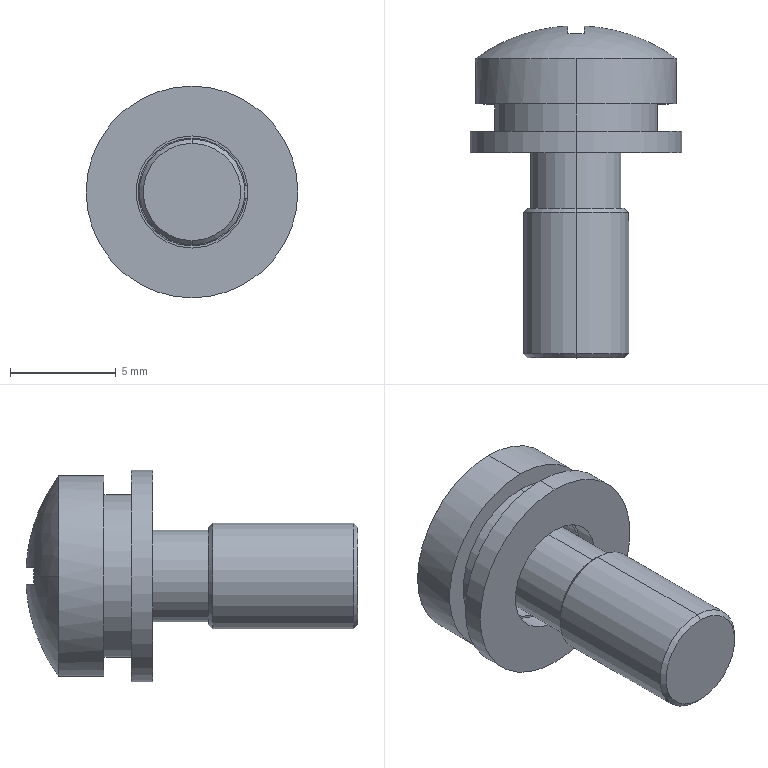Part | STEP file | 3 solids | 46 faces | box 10 x 15.681 x 10 mm | volume 491.081 mm3 | plane 22 | cylinder 16 | cone 4 | torus 2 | sphere 2 | commonest cylinder face diameters 5.1 x3 7.7 x3 4.33 x2 5 x2 5.3 x2 9.5 x2
STEP:
#1=CARTESIAN_POINT('',(0.,-15.7,-2.3));
#2=VERTEX_POINT('',#1);
#3=CARTESIAN_POINT('',(0.,-15.7,2.3));
#4=VERTEX_POINT('',#3);
#5=CARTESIAN_POINT('',(0.,-15.7,0.));
#6=DIRECTION('',(0.,-1.,0.));
#7=DIRECTION('',(0.,0.,1.));
#8=AXIS2_PLACEMENT_3D('',#5,#6,#7);
#9=CIRCLE('',#8,2.3);
#10=EDGE_CURVE('',#2,#4,#9,.T.);
#11=ORIENTED_EDGE('',*,*,#10,.F.);
#12=CARTESIAN_POINT('',(0.,-15.5,-2.5));
#13=VERTEX_POINT('',#12);
#14=CARTESIAN_POINT('',(0.,-15.7,-2.3));
#15=DIRECTION('',(0.,0.7071,-0.7071));
#16=VECTOR('',#15,1000.);
#17=LINE('',#14,#16);
#18=EDGE_CURVE('',#2,#13,#17,.T.);
#19=ORIENTED_EDGE('',*,*,#18,.T.);
#20=CARTESIAN_POINT('',(0.,-15.5,2.5));
#21=VERTEX_POINT('',#20);
#22=CARTESIAN_POINT('',(0.,-15.5,0.));
#23=DIRECTION('',(0.,1.,0.));
#24=DIRECTION('',(0.,0.,1.));
#25=AXIS2_PLACEMENT_3D('',#22,#23,#24);
#26=CIRCLE('',#25,2.5);
#27=EDGE_CURVE('',#21,#13,#26,.T.);
#28=ORIENTED_EDGE('',*,*,#27,.F.);
#29=CARTESIAN_POINT('',(0.,-15.7,2.3));
#30=DIRECTION('',(0.,0.7071,0.7071));
#31=VECTOR('',#30,1000.);
#32=LINE('',#29,#31);
#33=EDGE_CURVE('',#4,#21,#32,.T.);
#34=ORIENTED_EDGE('',*,*,#33,.F.);
#35=EDGE_LOOP('',(#11,#19,#28,#34));
#36=FACE_OUTER_BOUND('',#35,.T.);
#37=CARTESIAN_POINT('',(0.,-15.7,0.));
#38=DIRECTION('',(0.,1.,0.));
#39=DIRECTION('',(0.,0.,1.));
#40=AXIS2_PLACEMENT_3D('',#37,#38,#39);
#41=CONICAL_SURFACE('',#40,2.3,0.7854);
#42=ADVANCED_FACE('',(#36),#41,.T.);
#43=CARTESIAN_POINT('',(0.,-8.63,2.3));
#44=VERTEX_POINT('',#43);
#45=CARTESIAN_POINT('',(0.,-8.63,-2.3));
#46=VERTEX_POINT('',#45);
#47=CARTESIAN_POINT('',(0.,-8.63,0.));
#48=DIRECTION('',(0.,1.,0.));
#49=DIRECTION('',(0.,0.,1.));
#50=AXIS2_PLACEMENT_3D('',#47,#48,#49);
#51=CIRCLE('',#50,2.3);
#52=EDGE_CURVE('',#44,#46,#51,.T.);
#53=ORIENTED_EDGE('',*,*,#52,.F.);
#54=CARTESIAN_POINT('',(0.,-8.83,2.5));
#55=VERTEX_POINT('',#54);
#56=CARTESIAN_POINT('',(0.,-8.83,2.5));
#57=DIRECTION('',(0.,-0.7071,0.7071));
#58=VECTOR('',#57,1000.);
#59=LINE('',#56,#58);
#60=EDGE_CURVE('',#44,#55,#59,.T.);
#61=ORIENTED_EDGE('',*,*,#60,.T.);
#62=CARTESIAN_POINT('',(0.,-8.83,-2.5));
#63=VERTEX_POINT('',#62);
#64=CARTESIAN_POINT('',(0.,-8.83,0.));
#65=DIRECTION('',(0.,-1.,0.));
#66=DIRECTION('',(0.,0.,1.));
#67=AXIS2_PLACEMENT_3D('',#64,#65,#66);
#68=CIRCLE('',#67,2.5);
#69=EDGE_CURVE('',#63,#55,#68,.T.);
#70=ORIENTED_EDGE('',*,*,#69,.F.);
#71=CARTESIAN_POINT('',(0.,-8.83,-2.5));
#72=DIRECTION('',(0.,-0.7071,-0.7071));
#73=VECTOR('',#72,1000.);
#74=LINE('',#71,#73);
#75=EDGE_CURVE('',#46,#63,#74,.T.);
#76=ORIENTED_EDGE('',*,*,#75,.F.);
#77=EDGE_LOOP('',(#53,#61,#70,#76));
#78=FACE_OUTER_BOUND('',#77,.T.);
#79=CARTESIAN_POINT('',(0.,-8.83,0.));
#80=DIRECTION('',(0.,-1.,0.));
#81=DIRECTION('',(0.,0.,-1.));
#82=AXIS2_PLACEMENT_3D('',#79,#80,#81);
#83=CONICAL_SURFACE('',#82,2.5,0.7854);
#84=ADVANCED_FACE('',(#78),#83,.T.);
#85=CARTESIAN_POINT('',(0.,-3.9,2.165));
#86=VERTEX_POINT('',#85);
#87=CARTESIAN_POINT('',(0.,-3.9,-2.165));
#88=VERTEX_POINT('',#87);
#89=CARTESIAN_POINT('',(0.,-3.9,0.));
#90=DIRECTION('',(0.,-1.,0.));
#91=DIRECTION('',(0.,0.,-1.));
#92=AXIS2_PLACEMENT_3D('',#89,#90,#91);
#93=CIRCLE('',#92,2.165);
#94=EDGE_CURVE('',#86,#88,#93,.T.);
#95=ORIENTED_EDGE('',*,*,#94,.F.);
#96=CARTESIAN_POINT('',(0.,-3.7,2.365));
#97=VERTEX_POINT('',#96);
#98=CARTESIAN_POINT('',(0.,-3.9,2.365));
#99=DIRECTION('',(1.,0.,0.));
#100=DIRECTION('',(0.,0.,-1.));
#101=AXIS2_PLACEMENT_3D('',#98,#99,#100);
#102=CIRCLE('',#101,0.2);
#103=EDGE_CURVE('',#86,#97,#102,.T.);
#104=ORIENTED_EDGE('',*,*,#103,.T.);
#105=CARTESIAN_POINT('',(0.,-3.7,-2.365));
#106=VERTEX_POINT('',#105);
#107=CARTESIAN_POINT('',(0.,-3.7,0.));
#108=DIRECTION('',(0.,1.,0.));
#109=DIRECTION('',(0.,0.,-1.));
#110=AXIS2_PLACEMENT_3D('',#107,#108,#109);
#111=CIRCLE('',#110,2.365);
#112=EDGE_CURVE('',#106,#97,#111,.T.);
#113=ORIENTED_EDGE('',*,*,#112,.F.);
#114=CARTESIAN_POINT('',(0.,-3.9,-2.365));
#115=DIRECTION('',(-1.,0.,0.));
#116=DIRECTION('',(0.,0.,1.));
#117=AXIS2_PLACEMENT_3D('',#114,#115,#116);
#118=CIRCLE('',#117,0.2);
#119=EDGE_CURVE('',#88,#106,#118,.T.);
#120=ORIENTED_EDGE('',*,*,#119,.F.);
#121=EDGE_LOOP('',(#95,#104,#113,#120));
#122=FACE_OUTER_BOUND('',#121,.T.);
#123=CARTESIAN_POINT('',(0.,-3.9,0.));
#124=DIRECTION('',(0.,-1.,0.));
#125=DIRECTION('',(0.,0.,-1.));
#126=AXIS2_PLACEMENT_3D('',#123,#124,#125);
#127=TOROIDAL_SURFACE('',#126,2.365,0.2);
#128=ADVANCED_FACE('',(#122),#127,.F.);
#129=CARTESIAN_POINT('',(-2.45,-0.3844,0.));
#130=VERTEX_POINT('',#129);
#131=CARTESIAN_POINT('',(-2.45,-0.3941,0.385));
#132=VERTEX_POINT('',#131);
#133=CARTESIAN_POINT('',(-2.45,-8.,0.));
#134=DIRECTION('',(1.,0.,0.));
#135=DIRECTION('',(0.,0.,1.));
#136=AXIS2_PLACEMENT_3D('',#133,#134,#135);
#137=CIRCLE('',#136,7.616);
#138=EDGE_CURVE('',#130,#132,#137,.T.);
#139=ORIENTED_EDGE('',*,*,#138,.F.);
#140=CARTESIAN_POINT('',(-4.75,-1.563,0.));
#141=VERTEX_POINT('',#140);
#142=CARTESIAN_POINT('',(0.,-8.,0.));
#143=DIRECTION('',(0.,0.,1.));
#144=DIRECTION('',(1.,0.,0.));
#145=AXIS2_PLACEMENT_3D('',#142,#143,#144);
#146=CIRCLE('',#145,8.);
#147=EDGE_CURVE('',#130,#141,#146,.T.);
#148=ORIENTED_EDGE('',*,*,#147,.T.);
#149=CARTESIAN_POINT('',(0.,-1.563,4.75));
#150=VERTEX_POINT('',#149);
#151=CARTESIAN_POINT('',(0.,-1.563,0.));
#152=DIRECTION('',(0.,-1.,0.));
#153=DIRECTION('',(0.,0.,-1.));
#154=AXIS2_PLACEMENT_3D('',#151,#152,#153);
#155=CIRCLE('',#154,4.75);
#156=EDGE_CURVE('',#150,#141,#155,.T.);
#157=ORIENTED_EDGE('',*,*,#156,.F.);
#158=CARTESIAN_POINT('',(4.75,-1.563,0.));
#159=VERTEX_POINT('',#158);
#160=CARTESIAN_POINT('',(0.,-1.563,0.));
#161=DIRECTION('',(0.,-1.,0.));
#162=DIRECTION('',(0.,0.,-1.));
#163=AXIS2_PLACEMENT_3D('',#160,#161,#162);
#164=CIRCLE('',#163,4.75);
#165=EDGE_CURVE('',#159,#150,#164,.T.);
#166=ORIENTED_EDGE('',*,*,#165,.F.);
#167=CARTESIAN_POINT('',(2.45,-0.3844,0.));
#168=VERTEX_POINT('',#167);
#169=CARTESIAN_POINT('',(0.,-8.,0.));
#170=DIRECTION('',(0.,0.,-1.));
#171=DIRECTION('',(-1.,0.,0.));
#172=AXIS2_PLACEMENT_3D('',#169,#170,#171);
#173=CIRCLE('',#172,8.);
#174=EDGE_CURVE('',#168,#159,#173,.T.);
#175=ORIENTED_EDGE('',*,*,#174,.F.);
#176=CARTESIAN_POINT('',(2.45,-0.3941,0.385));
#177=VERTEX_POINT('',#176);
#178=CARTESIAN_POINT('',(2.45,-8.,0.));
#179=DIRECTION('',(-1.,0.,0.));
#180=DIRECTION('',(0.,0.,-1.));
#181=AXIS2_PLACEMENT_3D('',#178,#179,#180);
#182=CIRCLE('',#181,7.616);
#183=EDGE_CURVE('',#177,#168,#182,.T.);
#184=ORIENTED_EDGE('',*,*,#183,.F.);
#185=CARTESIAN_POINT('',(0.385,-0.01855,0.385));
#186=VERTEX_POINT('',#185);
#187=CARTESIAN_POINT('',(0.,-8.,0.385));
#188=DIRECTION('',(0.,0.,-1.));
#189=DIRECTION('',(1.,0.,0.));
#190=AXIS2_PLACEMENT_3D('',#187,#188,#189);
#191=CIRCLE('',#190,7.991);
#192=EDGE_CURVE('',#186,#177,#191,.T.);
#193=ORIENTED_EDGE('',*,*,#192,.F.);
#194=CARTESIAN_POINT('',(0.385,-0.3941,2.45));
#195=VERTEX_POINT('',#194);
#196=CARTESIAN_POINT('',(0.385,-8.,0.));
#197=DIRECTION('',(-1.,0.,0.));
#198=DIRECTION('',(0.,0.,-1.));
#199=AXIS2_PLACEMENT_3D('',#196,#197,#198);
#200=CIRCLE('',#199,7.991);
#201=EDGE_CURVE('',#195,#186,#200,.T.);
#202=ORIENTED_EDGE('',*,*,#201,.F.);
#203=CARTESIAN_POINT('',(-0.385,-0.3941,2.45));
#204=VERTEX_POINT('',#203);
#205=CARTESIAN_POINT('',(0.,-8.,2.45));
#206=DIRECTION('',(0.,0.,-1.));
#207=DIRECTION('',(1.,0.,0.));
#208=AXIS2_PLACEMENT_3D('',#205,#206,#207);
#209=CIRCLE('',#208,7.616);
#210=EDGE_CURVE('',#204,#195,#209,.T.);
#211=ORIENTED_EDGE('',*,*,#210,.F.);
#212=CARTESIAN_POINT('',(-0.385,-0.01855,0.385));
#213=VERTEX_POINT('',#212);
#214=CARTESIAN_POINT('',(-0.385,-8.,0.));
#215=DIRECTION('',(1.,0.,0.));
#216=DIRECTION('',(0.,0.,1.));
#217=AXIS2_PLACEMENT_3D('',#214,#215,#216);
#218=CIRCLE('',#217,7.991);
#219=EDGE_CURVE('',#213,#204,#218,.T.);
#220=ORIENTED_EDGE('',*,*,#219,.F.);
#221=CARTESIAN_POINT('',(0.,-8.,0.385));
#222=DIRECTION('',(0.,0.,-1.));
#223=DIRECTION('',(1.,0.,0.));
#224=AXIS2_PLACEMENT_3D('',#221,#222,#223);
#225=CIRCLE('',#224,7.991);
#226=EDGE_CURVE('',#132,#213,#225,.T.);
#227=ORIENTED_EDGE('',*,*,#226,.F.);
#228=EDGE_LOOP('',(#139,#148,#157,#166,#175,#184,#193,#202,#211,#220,#227));
#229=FACE_OUTER_BOUND('',#228,.T.);
#230=CARTESIAN_POINT('',(0.,-8.,0.));
#231=DIRECTION('',(0.,0.,1.));
#232=DIRECTION('',(1.,0.,0.));
#233=AXIS2_PLACEMENT_3D('',#230,#231,#232);
#234=SPHERICAL_SURFACE('',#233,8.);
#235=ADVANCED_FACE('',(#229),#234,.T.);
#236=CARTESIAN_POINT('',(0.,-1.563,-4.75));
#237=VERTEX_POINT('',#236);
#238=CARTESIAN_POINT('',(0.,-1.563,0.));
#239=DIRECTION('',(0.,-1.,0.));
#240=DIRECTION('',(0.,0.,-1.));
#241=AXIS2_PLACEMENT_3D('',#238,#239,#240);
#242=CIRCLE('',#241,4.75);
#243=EDGE_CURVE('',#237,#159,#242,.T.);
#244=ORIENTED_EDGE('',*,*,#243,.T.);
#245=ORIENTED_EDGE('',*,*,#165,.T.);
#246=CARTESIAN_POINT('',(0.,-3.7,4.75));
#247=VERTEX_POINT('',#246);
#248=CARTESIAN_POINT('',(0.,-15.7,4.75));
#249=DIRECTION('',(0.,-1.,0.));
#250=VECTOR('',#249,1000.);
#251=LINE('',#248,#250);
#252=EDGE_CURVE('',#150,#247,#251,.T.);
#253=ORIENTED_EDGE('',*,*,#252,.T.);
#254=CARTESIAN_POINT('',(0.,-3.7,-4.75));
#255=VERTEX_POINT('',#254);
#256=CARTESIAN_POINT('',(0.,-3.7,0.));
#257=DIRECTION('',(0.,-1.,0.));
#258=DIRECTION('',(0.,0.,-1.));
#259=AXIS2_PLACEMENT_3D('',#256,#257,#258);
#260=CIRCLE('',#259,4.75);
#261=EDGE_CURVE('',#255,#247,#260,.T.);
#262=ORIENTED_EDGE('',*,*,#261,.F.);
#263=CARTESIAN_POINT('',(0.,-15.7,-4.75));
#264=DIRECTION('',(0.,-1.,0.));
#265=VECTOR('',#264,1000.);
#266=LINE('',#263,#265);
#267=EDGE_CURVE('',#237,#255,#266,.T.);
#268=ORIENTED_EDGE('',*,*,#267,.F.);
#269=EDGE_LOOP('',(#244,#245,#253,#262,#268));
#270=FACE_OUTER_BOUND('',#269,.T.);
#271=CARTESIAN_POINT('',(0.,-15.7,0.));
#272=DIRECTION('',(0.,-1.,0.));
#273=DIRECTION('',(0.,0.,-1.));
#274=AXIS2_PLACEMENT_3D('',#271,#272,#273);
#275=CYLINDRICAL_SURFACE('',#274,4.75);
#276=ADVANCED_FACE('',(#270),#275,.T.);
#277=CARTESIAN_POINT('',(0.,-3.9,0.));
#278=DIRECTION('',(0.,-1.,0.));
#279=DIRECTION('',(0.,0.,-1.));
#280=AXIS2_PLACEMENT_3D('',#277,#278,#279);
#281=CIRCLE('',#280,2.165);
#282=EDGE_CURVE('',#88,#86,#281,.T.);
#283=ORIENTED_EDGE('',*,*,#282,.T.);
#284=CARTESIAN_POINT('',(0.,-8.63,2.165));
#285=VERTEX_POINT('',#284);
#286=CARTESIAN_POINT('',(0.,-15.7,2.165));
#287=DIRECTION('',(0.,-1.,0.));
#288=VECTOR('',#287,1000.);
#289=LINE('',#286,#288);
#290=EDGE_CURVE('',#86,#285,#289,.T.);
#291=ORIENTED_EDGE('',*,*,#290,.T.);
#292=CARTESIAN_POINT('',(0.,-8.63,-2.165));
#293=VERTEX_POINT('',#292);
#294=CARTESIAN_POINT('',(0.,-8.63,0.));
#295=DIRECTION('',(0.,-1.,0.));
#296=DIRECTION('',(0.,0.,-1.));
#297=AXIS2_PLACEMENT_3D('',#294,#295,#296);
#298=CIRCLE('',#297,2.165);
#299=EDGE_CURVE('',#293,#285,#298,.T.);
#300=ORIENTED_EDGE('',*,*,#299,.F.);
#301=CARTESIAN_POINT('',(0.,-15.7,-2.165));
#302=DIRECTION('',(0.,-1.,0.));
#303=VECTOR('',#302,1000.);
#304=LINE('',#301,#303);
#305=EDGE_CURVE('',#88,#293,#304,.T.);
#306=ORIENTED_EDGE('',*,*,#305,.F.);
#307=EDGE_LOOP('',(#283,#291,#300,#306));
#308=FACE_OUTER_BOUND('',#307,.T.);
#309=CARTESIAN_POINT('',(0.,-15.7,0.));
#310=DIRECTION('',(0.,-1.,0.));
#311=DIRECTION('',(0.,0.,-1.));
#312=AXIS2_PLACEMENT_3D('',#309,#310,#311);
#313=CYLINDRICAL_SURFACE('',#312,2.165);
#314=ADVANCED_FACE('',(#308),#313,.T.);
#315=ORIENTED_EDGE('',*,*,#69,.T.);
#316=CARTESIAN_POINT('',(0.,-15.7,2.5));
#317=DIRECTION('',(0.,-1.,0.));
#318=VECTOR('',#317,1000.);
#319=LINE('',#316,#318);
#320=EDGE_CURVE('',#55,#21,#319,.T.);
#321=ORIENTED_EDGE('',*,*,#320,.T.);
#322=ORIENTED_EDGE('',*,*,#27,.T.);
#323=CARTESIAN_POINT('',(0.,-15.7,-2.5));
#324=DIRECTION('',(0.,-1.,0.));
#325=VECTOR('',#324,1000.);
#326=LINE('',#323,#325);
#327=EDGE_CURVE('',#63,#13,#326,.T.);
#328=ORIENTED_EDGE('',*,*,#327,.F.);
#329=EDGE_LOOP('',(#315,#321,#322,#328));
#330=FACE_OUTER_BOUND('',#329,.T.);
#331=CARTESIAN_POINT('',(0.,-15.7,0.));
#332=DIRECTION('',(0.,-1.,0.));
#333=DIRECTION('',(0.,0.,-1.));
#334=AXIS2_PLACEMENT_3D('',#331,#332,#333);
#335=CYLINDRICAL_SURFACE('',#334,2.5);
#336=ADVANCED_FACE('',(#330),#335,.T.);
#337=CARTESIAN_POINT('',(0.,-15.7,0.));
#338=DIRECTION('',(0.,-1.,0.));
#339=DIRECTION('',(0.,0.,1.));
#340=AXIS2_PLACEMENT_3D('',#337,#338,#339);
#341=CIRCLE('',#340,2.3);
#342=EDGE_CURVE('',#4,#2,#341,.T.);
#343=ORIENTED_EDGE('',*,*,#342,.T.);
#344=ORIENTED_EDGE('',*,*,#10,.T.);
#345=EDGE_LOOP('',(#343,#344));
#346=FACE_OUTER_BOUND('',#345,.T.);
#347=CARTESIAN_POINT('',(0.,-15.7,0.));
#348=DIRECTION('',(0.,1.,0.));
#349=DIRECTION('',(0.,0.,1.));
#350=AXIS2_PLACEMENT_3D('',#347,#348,#349);
#351=PLANE('',#350);
#352=ADVANCED_FACE('',(#346),#351,.F.);
#353=ORIENTED_EDGE('',*,*,#320,.F.);
#354=CARTESIAN_POINT('',(0.,-8.83,0.));
#355=DIRECTION('',(0.,-1.,0.));
#356=DIRECTION('',(0.,0.,1.));
#357=AXIS2_PLACEMENT_3D('',#354,#355,#356);
#358=CIRCLE('',#357,2.5);
#359=EDGE_CURVE('',#55,#63,#358,.T.);
#360=ORIENTED_EDGE('',*,*,#359,.T.);
#361=ORIENTED_EDGE('',*,*,#327,.T.);
#362=CARTESIAN_POINT('',(0.,-15.5,0.));
#363=DIRECTION('',(0.,1.,0.));
#364=DIRECTION('',(0.,0.,1.));
#365=AXIS2_PLACEMENT_3D('',#362,#363,#364);
#366=CIRCLE('',#365,2.5);
#367=EDGE_CURVE('',#13,#21,#366,.T.);
#368=ORIENTED_EDGE('',*,*,#367,.T.);
#369=EDGE_LOOP('',(#353,#360,#361,#368));
#370=FACE_OUTER_BOUND('',#369,.T.);
#371=CARTESIAN_POINT('',(0.,-15.7,0.));
#372=DIRECTION('',(0.,-1.,0.));
#373=DIRECTION('',(0.,0.,-1.));
#374=AXIS2_PLACEMENT_3D('',#371,#372,#373);
#375=CYLINDRICAL_SURFACE('',#374,2.5);
#376=ADVANCED_FACE('',(#370),#375,.T.);
#377=CARTESIAN_POINT('',(0.,-8.63,0.));
#378=DIRECTION('',(0.,1.,0.));
#379=DIRECTION('',(0.,0.,1.));
#380=AXIS2_PLACEMENT_3D('',#377,#378,#379);
#381=CIRCLE('',#380,2.3);
#382=EDGE_CURVE('',#46,#44,#381,.T.);
#383=ORIENTED_EDGE('',*,*,#382,.T.);
#384=ORIENTED_EDGE('',*,*,#52,.T.);
#385=EDGE_LOOP('',(#383,#384));
#386=FACE_OUTER_BOUND('',#385,.T.);
#387=ORIENTED_EDGE('',*,*,#299,.T.);
#388=CARTESIAN_POINT('',(0.,-8.63,0.));
#389=DIRECTION('',(0.,-1.,0.));
#390=DIRECTION('',(0.,0.,-1.));
#391=AXIS2_PLACEMENT_3D('',#388,#389,#390);
#392=CIRCLE('',#391,2.165);
#393=EDGE_CURVE('',#285,#293,#392,.T.);
#394=ORIENTED_EDGE('',*,*,#393,.T.);
#395=EDGE_LOOP('',(#387,#394));
#396=FACE_BOUND('',#395,.T.);
#397=CARTESIAN_POINT('',(0.,-8.63,0.));
#398=DIRECTION('',(0.,1.,0.));
#399=DIRECTION('',(0.,0.,1.));
#400=AXIS2_PLACEMENT_3D('',#397,#398,#399);
#401=PLANE('',#400);
#402=ADVANCED_FACE('',(#386,#396),#401,.T.);
#403=ORIENTED_EDGE('',*,*,#290,.F.);
#404=ORIENTED_EDGE('',*,*,#94,.T.);
#405=ORIENTED_EDGE('',*,*,#305,.T.);
#406=ORIENTED_EDGE('',*,*,#393,.F.);
#407=EDGE_LOOP('',(#403,#404,#405,#406));
#408=FACE_OUTER_BOUND('',#407,.T.);
#409=CARTESIAN_POINT('',(0.,-15.7,0.));
#410=DIRECTION('',(0.,-1.,0.));
#411=DIRECTION('',(0.,0.,-1.));
#412=AXIS2_PLACEMENT_3D('',#409,#410,#411);
#413=CYLINDRICAL_SURFACE('',#412,2.165);
#414=ADVANCED_FACE('',(#408),#413,.T.);
#415=ORIENTED_EDGE('',*,*,#112,.T.);
#416=CARTESIAN_POINT('',(0.,-3.7,0.));
#417=DIRECTION('',(0.,1.,0.));
#418=DIRECTION('',(0.,0.,-1.));
#419=AXIS2_PLACEMENT_3D('',#416,#417,#418);
#420=CIRCLE('',#419,2.365);
#421=EDGE_CURVE('',#97,#106,#420,.T.);
#422=ORIENTED_EDGE('',*,*,#421,.T.);
#423=EDGE_LOOP('',(#415,#422));
#424=FACE_BOUND('',#423,.T.);
#425=ORIENTED_EDGE('',*,*,#261,.T.);
#426=CARTESIAN_POINT('',(0.,-3.7,0.));
#427=DIRECTION('',(0.,-1.,0.));
#428=DIRECTION('',(0.,0.,-1.));
#429=AXIS2_PLACEMENT_3D('',#426,#427,#428);
#430=CIRCLE('',#429,4.75);
#431=EDGE_CURVE('',#247,#255,#430,.T.);
#432=ORIENTED_EDGE('',*,*,#431,.T.);
#433=EDGE_LOOP('',(#425,#432));
#434=FACE_OUTER_BOUND('',#433,.T.);
#435=CARTESIAN_POINT('',(0.,-3.7,0.));
#436=DIRECTION('',(0.,-1.,0.));
#437=DIRECTION('',(0.,0.,-1.));
#438=AXIS2_PLACEMENT_3D('',#435,#436,#437);
#439=PLANE('',#438);
#440=ADVANCED_FACE('',(#424,#434),#439,.T.);
#441=ORIENTED_EDGE('',*,*,#252,.F.);
#442=ORIENTED_EDGE('',*,*,#156,.T.);
#443=CARTESIAN_POINT('',(0.,-1.563,0.));
#444=DIRECTION('',(0.,-1.,0.));
#445=DIRECTION('',(0.,0.,-1.));
#446=AXIS2_PLACEMENT_3D('',#443,#444,#445);
#447=CIRCLE('',#446,4.75);
#448=EDGE_CURVE('',#141,#237,#447,.T.);
#449=ORIENTED_EDGE('',*,*,#448,.T.);
#450=ORIENTED_EDGE('',*,*,#267,.T.);
#451=ORIENTED_EDGE('',*,*,#431,.F.);
#452=EDGE_LOOP('',(#441,#442,#449,#450,#451));
#453=FACE_OUTER_BOUND('',#452,.T.);
#454=CARTESIAN_POINT('',(0.,-15.7,0.));
#455=DIRECTION('',(0.,-1.,0.));
#456=DIRECTION('',(0.,0.,-1.));
#457=AXIS2_PLACEMENT_3D('',#454,#455,#456);
#458=CYLINDRICAL_SURFACE('',#457,4.75);
#459=ADVANCED_FACE('',(#453),#458,.T.);
#460=ORIENTED_EDGE('',*,*,#147,.F.);
#461=CARTESIAN_POINT('',(-2.45,-0.3941,-0.385));
#462=VERTEX_POINT('',#461);
#463=CARTESIAN_POINT('',(-2.45,-8.,0.));
#464=DIRECTION('',(1.,0.,0.));
#465=DIRECTION('',(0.,0.,1.));
#466=AXIS2_PLACEMENT_3D('',#463,#464,#465);
#467=CIRCLE('',#466,7.616);
#468=EDGE_CURVE('',#462,#130,#467,.T.);
#469=ORIENTED_EDGE('',*,*,#468,.F.);
#470=CARTESIAN_POINT('',(-0.385,-0.01855,-0.385));
#471=VERTEX_POINT('',#470);
#472=CARTESIAN_POINT('',(0.,-8.,-0.385));
#473=DIRECTION('',(0.,0.,1.));
#474=DIRECTION('',(-1.,0.,0.));
#475=AXIS2_PLACEMENT_3D('',#472,#473,#474);
#476=CIRCLE('',#475,7.991);
#477=EDGE_CURVE('',#471,#462,#476,.T.);
#478=ORIENTED_EDGE('',*,*,#477,.F.);
#479=CARTESIAN_POINT('',(-0.385,-0.3941,-2.45));
#480=VERTEX_POINT('',#479);
#481=CARTESIAN_POINT('',(-0.385,-8.,0.));
#482=DIRECTION('',(1.,0.,0.));
#483=DIRECTION('',(0.,0.,1.));
#484=AXIS2_PLACEMENT_3D('',#481,#482,#483);
#485=CIRCLE('',#484,7.991);
#486=EDGE_CURVE('',#480,#471,#485,.T.);
#487=ORIENTED_EDGE('',*,*,#486,.F.);
#488=CARTESIAN_POINT('',(0.385,-0.3941,-2.45));
#489=VERTEX_POINT('',#488);
#490=CARTESIAN_POINT('',(0.,-8.,-2.45));
#491=DIRECTION('',(0.,0.,1.));
#492=DIRECTION('',(-1.,0.,0.));
#493=AXIS2_PLACEMENT_3D('',#490,#491,#492);
#494=CIRCLE('',#493,7.616);
#495=EDGE_CURVE('',#489,#480,#494,.T.);
#496=ORIENTED_EDGE('',*,*,#495,.F.);
#497=CARTESIAN_POINT('',(0.385,-0.01855,-0.385));
#498=VERTEX_POINT('',#497);
#499=CARTESIAN_POINT('',(0.385,-8.,0.));
#500=DIRECTION('',(-1.,0.,0.));
#501=DIRECTION('',(0.,0.,-1.));
#502=AXIS2_PLACEMENT_3D('',#499,#500,#501);
#503=CIRCLE('',#502,7.991);
#504=EDGE_CURVE('',#498,#489,#503,.T.);
#505=ORIENTED_EDGE('',*,*,#504,.F.);
#506=CARTESIAN_POINT('',(2.45,-0.3941,-0.385));
#507=VERTEX_POINT('',#506);
#508=CARTESIAN_POINT('',(0.,-8.,-0.385));
#509=DIRECTION('',(0.,0.,1.));
#510=DIRECTION('',(-1.,0.,0.));
#511=AXIS2_PLACEMENT_3D('',#508,#509,#510);
#512=CIRCLE('',#511,7.991);
#513=EDGE_CURVE('',#507,#498,#512,.T.);
#514=ORIENTED_EDGE('',*,*,#513,.F.);
#515=CARTESIAN_POINT('',(2.45,-8.,0.));
#516=DIRECTION('',(-1.,0.,0.));
#517=DIRECTION('',(0.,0.,-1.));
#518=AXIS2_PLACEMENT_3D('',#515,#516,#517);
#519=CIRCLE('',#518,7.616);
#520=EDGE_CURVE('',#168,#507,#519,.T.);
#521=ORIENTED_EDGE('',*,*,#520,.F.);
#522=ORIENTED_EDGE('',*,*,#174,.T.);
#523=ORIENTED_EDGE('',*,*,#243,.F.);
#524=ORIENTED_EDGE('',*,*,#448,.F.);
#525=EDGE_LOOP('',(#460,#469,#478,#487,#496,#505,#514,#521,#522,#523,#524));
#526=FACE_OUTER_BOUND('',#525,.T.);
#527=CARTESIAN_POINT('',(0.,-8.,0.));
#528=DIRECTION('',(0.,0.,1.));
#529=DIRECTION('',(1.,0.,0.));
#530=AXIS2_PLACEMENT_3D('',#527,#528,#529);
#531=SPHERICAL_SURFACE('',#530,8.);
#532=ADVANCED_FACE('',(#526),#531,.T.);
#533=ORIENTED_EDGE('',*,*,#513,.T.);
#534=CARTESIAN_POINT('',(0.385,-2.74,-0.385));
#535=VERTEX_POINT('',#534);
#536=CARTESIAN_POINT('',(0.385,-2.74,-0.385));
#537=DIRECTION('',(0.,1.,0.));
#538=VECTOR('',#537,1000.);
#539=LINE('',#536,#538);
#540=EDGE_CURVE('',#535,#498,#539,.T.);
#541=ORIENTED_EDGE('',*,*,#540,.F.);
#542=CARTESIAN_POINT('',(2.45,-2.74,-0.385));
#543=VERTEX_POINT('',#542);
#544=CARTESIAN_POINT('',(0.385,-2.74,-0.385));
#545=DIRECTION('',(-1.,0.,0.));
#546=VECTOR('',#545,1000.);
#547=LINE('',#544,#546);
#548=EDGE_CURVE('',#543,#535,#547,.T.);
#549=ORIENTED_EDGE('',*,*,#548,.F.);
#550=CARTESIAN_POINT('',(2.45,-2.74,-0.385));
#551=DIRECTION('',(0.,1.,0.));
#552=VECTOR('',#551,1000.);
#553=LINE('',#550,#552);
#554=EDGE_CURVE('',#543,#507,#553,.T.);
#555=ORIENTED_EDGE('',*,*,#554,.T.);
#556=EDGE_LOOP('',(#533,#541,#549,#555));
#557=FACE_OUTER_BOUND('',#556,.T.);
#558=CARTESIAN_POINT('',(0.385,-2.74,-0.385));
#559=DIRECTION('',(0.,0.,-1.));
#560=DIRECTION('',(-1.,0.,0.));
#561=AXIS2_PLACEMENT_3D('',#558,#559,#560);
#562=PLANE('',#561);
#563=ADVANCED_FACE('',(#557),#562,.F.);
#564=ORIENTED_EDGE('',*,*,#183,.T.);
#565=ORIENTED_EDGE('',*,*,#520,.T.);
#566=ORIENTED_EDGE('',*,*,#554,.F.);
#567=CARTESIAN_POINT('',(2.45,-2.74,0.385));
#568=VERTEX_POINT('',#567);
#569=CARTESIAN_POINT('',(2.45,-2.74,-0.385));
#570=DIRECTION('',(0.,0.,-1.));
#571=VECTOR('',#570,1000.);
#572=LINE('',#569,#571);
#573=EDGE_CURVE('',#568,#543,#572,.T.);
#574=ORIENTED_EDGE('',*,*,#573,.F.);
#575=CARTESIAN_POINT('',(2.45,-2.74,0.385));
#576=DIRECTION('',(0.,1.,0.));
#577=VECTOR('',#576,1000.);
#578=LINE('',#575,#577);
#579=EDGE_CURVE('',#568,#177,#578,.T.);
#580=ORIENTED_EDGE('',*,*,#579,.T.);
#581=EDGE_LOOP('',(#564,#565,#566,#574,#580));
#582=FACE_OUTER_BOUND('',#581,.T.);
#583=CARTESIAN_POINT('',(2.45,-2.74,-0.385));
#584=DIRECTION('',(1.,0.,0.));
#585=DIRECTION('',(0.,0.,-1.));
#586=AXIS2_PLACEMENT_3D('',#583,#584,#585);
#587=PLANE('',#586);
#588=ADVANCED_FACE('',(#582),#587,.F.);
#589=ORIENTED_EDGE('',*,*,#192,.T.);
#590=ORIENTED_EDGE('',*,*,#579,.F.);
#591=CARTESIAN_POINT('',(0.385,-2.74,0.385));
#592=VERTEX_POINT('',#591);
#593=CARTESIAN_POINT('',(0.385,-2.74,0.385));
#594=DIRECTION('',(1.,0.,0.));
#595=VECTOR('',#594,1000.);
#596=LINE('',#593,#595);
#597=EDGE_CURVE('',#592,#568,#596,.T.);
#598=ORIENTED_EDGE('',*,*,#597,.F.);
#599=CARTESIAN_POINT('',(0.385,-2.74,0.385));
#600=DIRECTION('',(0.,1.,0.));
#601=VECTOR('',#600,1000.);
#602=LINE('',#599,#601);
#603=EDGE_CURVE('',#592,#186,#602,.T.);
#604=ORIENTED_EDGE('',*,*,#603,.T.);
#605=EDGE_LOOP('',(#589,#590,#598,#604));
#606=FACE_OUTER_BOUND('',#605,.T.);
#607=CARTESIAN_POINT('',(0.385,-2.74,0.385));
#608=DIRECTION('',(0.,0.,1.));
#609=DIRECTION('',(1.,0.,0.));
#610=AXIS2_PLACEMENT_3D('',#607,#608,#609);
#611=PLANE('',#610);
#612=ADVANCED_FACE('',(#606),#611,.F.);
#613=ORIENTED_EDGE('',*,*,#201,.T.);
#614=ORIENTED_EDGE('',*,*,#603,.F.);
#615=CARTESIAN_POINT('',(0.385,-2.74,2.45));
#616=VERTEX_POINT('',#615);
#617=CARTESIAN_POINT('',(0.385,-2.74,2.45));
#618=DIRECTION('',(0.,0.,-1.));
#619=VECTOR('',#618,1000.);
#620=LINE('',#617,#619);
#621=EDGE_CURVE('',#616,#592,#620,.T.);
#622=ORIENTED_EDGE('',*,*,#621,.F.);
#623=CARTESIAN_POINT('',(0.385,-2.74,2.45));
#624=DIRECTION('',(0.,1.,0.));
#625=VECTOR('',#624,1000.);
#626=LINE('',#623,#625);
#627=EDGE_CURVE('',#616,#195,#626,.T.);
#628=ORIENTED_EDGE('',*,*,#627,.T.);
#629=EDGE_LOOP('',(#613,#614,#622,#628));
#630=FACE_OUTER_BOUND('',#629,.T.);
#631=CARTESIAN_POINT('',(0.385,-2.74,2.45));
#632=DIRECTION('',(1.,0.,0.));
#633=DIRECTION('',(0.,0.,-1.));
#634=AXIS2_PLACEMENT_3D('',#631,#632,#633);
#635=PLANE('',#634);
#636=ADVANCED_FACE('',(#630),#635,.F.);
#637=ORIENTED_EDGE('',*,*,#210,.T.);
#638=ORIENTED_EDGE('',*,*,#627,.F.);
#639=CARTESIAN_POINT('',(-0.385,-2.74,2.45));
#640=VERTEX_POINT('',#639);
#641=CARTESIAN_POINT('',(-0.385,-2.74,2.45));
#642=DIRECTION('',(1.,0.,0.));
#643=VECTOR('',#642,1000.);
#644=LINE('',#641,#643);
#645=EDGE_CURVE('',#640,#616,#644,.T.);
#646=ORIENTED_EDGE('',*,*,#645,.F.);
#647=CARTESIAN_POINT('',(-0.385,-2.74,2.45));
#648=DIRECTION('',(0.,1.,0.));
#649=VECTOR('',#648,1000.);
#650=LINE('',#647,#649);
#651=EDGE_CURVE('',#640,#204,#650,.T.);
#652=ORIENTED_EDGE('',*,*,#651,.T.);
#653=EDGE_LOOP('',(#637,#638,#646,#652));
#654=FACE_OUTER_BOUND('',#653,.T.);
#655=CARTESIAN_POINT('',(-0.385,-2.74,2.45));
#656=DIRECTION('',(0.,0.,1.));
#657=DIRECTION('',(1.,0.,0.));
#658=AXIS2_PLACEMENT_3D('',#655,#656,#657);
#659=PLANE('',#658);
#660=ADVANCED_FACE('',(#654),#659,.F.);
#661=ORIENTED_EDGE('',*,*,#219,.T.);
#662=ORIENTED_EDGE('',*,*,#651,.F.);
#663=CARTESIAN_POINT('',(-0.385,-2.74,0.385));
#664=VERTEX_POINT('',#663);
#665=CARTESIAN_POINT('',(-0.385,-2.74,2.45));
#666=DIRECTION('',(0.,0.,1.));
#667=VECTOR('',#666,1000.);
#668=LINE('',#665,#667);
#669=EDGE_CURVE('',#664,#640,#668,.T.);
#670=ORIENTED_EDGE('',*,*,#669,.F.);
#671=CARTESIAN_POINT('',(-0.385,-2.74,0.385));
#672=DIRECTION('',(0.,1.,0.));
#673=VECTOR('',#672,1000.);
#674=LINE('',#671,#673);
#675=EDGE_CURVE('',#664,#213,#674,.T.);
#676=ORIENTED_EDGE('',*,*,#675,.T.);
#677=EDGE_LOOP('',(#661,#662,#670,#676));
#678=FACE_OUTER_BOUND('',#677,.T.);
#679=CARTESIAN_POINT('',(-0.385,-2.74,2.45));
#680=DIRECTION('',(-1.,0.,0.));
#681=DIRECTION('',(0.,0.,1.));
#682=AXIS2_PLACEMENT_3D('',#679,#680,#681);
#683=PLANE('',#682);
#684=ADVANCED_FACE('',(#678),#683,.F.);
#685=ORIENTED_EDGE('',*,*,#226,.T.);
#686=ORIENTED_EDGE('',*,*,#675,.F.);
#687=CARTESIAN_POINT('',(-2.45,-2.74,0.385));
#688=VERTEX_POINT('',#687);
#689=CARTESIAN_POINT('',(-0.385,-2.74,0.385));
#690=DIRECTION('',(1.,0.,0.));
#691=VECTOR('',#690,1000.);
#692=LINE('',#689,#691);
#693=EDGE_CURVE('',#688,#664,#692,.T.);
#694=ORIENTED_EDGE('',*,*,#693,.F.);
#695=CARTESIAN_POINT('',(-2.45,-2.74,0.385));
#696=DIRECTION('',(0.,1.,0.));
#697=VECTOR('',#696,1000.);
#698=LINE('',#695,#697);
#699=EDGE_CURVE('',#688,#132,#698,.T.);
#700=ORIENTED_EDGE('',*,*,#699,.T.);
#701=EDGE_LOOP('',(#685,#686,#694,#700));
#702=FACE_OUTER_BOUND('',#701,.T.);
#703=CARTESIAN_POINT('',(-0.385,-2.74,0.385));
#704=DIRECTION('',(0.,0.,1.));
#705=DIRECTION('',(1.,0.,0.));
#706=AXIS2_PLACEMENT_3D('',#703,#704,#705);
#707=PLANE('',#706);
#708=ADVANCED_FACE('',(#702),#707,.F.);
#709=ORIENTED_EDGE('',*,*,#468,.T.);
#710=ORIENTED_EDGE('',*,*,#138,.T.);
#711=ORIENTED_EDGE('',*,*,#699,.F.);
#712=CARTESIAN_POINT('',(-2.45,-2.74,-0.385));
#713=VERTEX_POINT('',#712);
#714=CARTESIAN_POINT('',(-2.45,-2.74,-0.385));
#715=DIRECTION('',(0.,0.,1.));
#716=VECTOR('',#715,1000.);
#717=LINE('',#714,#716);
#718=EDGE_CURVE('',#713,#688,#717,.T.);
#719=ORIENTED_EDGE('',*,*,#718,.F.);
#720=CARTESIAN_POINT('',(-2.45,-2.74,-0.385));
#721=DIRECTION('',(0.,1.,0.));
#722=VECTOR('',#721,1000.);
#723=LINE('',#720,#722);
#724=EDGE_CURVE('',#713,#462,#723,.T.);
#725=ORIENTED_EDGE('',*,*,#724,.T.);
#726=EDGE_LOOP('',(#709,#710,#711,#719,#725));
#727=FACE_OUTER_BOUND('',#726,.T.);
#728=CARTESIAN_POINT('',(-2.45,-2.74,-0.385));
#729=DIRECTION('',(-1.,0.,0.));
#730=DIRECTION('',(0.,0.,1.));
#731=AXIS2_PLACEMENT_3D('',#728,#729,#730);
#732=PLANE('',#731);
#733=ADVANCED_FACE('',(#727),#732,.F.);
#734=ORIENTED_EDGE('',*,*,#477,.T.);
#735=ORIENTED_EDGE('',*,*,#724,.F.);
#736=CARTESIAN_POINT('',(-0.385,-2.74,-0.385));
#737=VERTEX_POINT('',#736);
#738=CARTESIAN_POINT('',(-0.385,-2.74,-0.385));
#739=DIRECTION('',(-1.,0.,0.));
#740=VECTOR('',#739,1000.);
#741=LINE('',#738,#740);
#742=EDGE_CURVE('',#737,#713,#741,.T.);
#743=ORIENTED_EDGE('',*,*,#742,.F.);
#744=CARTESIAN_POINT('',(-0.385,-2.74,-0.385));
#745=DIRECTION('',(0.,1.,0.));
#746=VECTOR('',#745,1000.);
#747=LINE('',#744,#746);
#748=EDGE_CURVE('',#737,#471,#747,.T.);
#749=ORIENTED_EDGE('',*,*,#748,.T.);
#750=EDGE_LOOP('',(#734,#735,#743,#749));
#751=FACE_OUTER_BOUND('',#750,.T.);
#752=CARTESIAN_POINT('',(-0.385,-2.74,-0.385));
#753=DIRECTION('',(0.,0.,-1.));
#754=DIRECTION('',(-1.,0.,0.));
#755=AXIS2_PLACEMENT_3D('',#752,#753,#754);
#756=PLANE('',#755);
#757=ADVANCED_FACE('',(#751),#756,.F.);
#758=ORIENTED_EDGE('',*,*,#486,.T.);
#759=ORIENTED_EDGE('',*,*,#748,.F.);
#760=CARTESIAN_POINT('',(-0.385,-2.74,-2.45));
#761=VERTEX_POINT('',#760);
#762=CARTESIAN_POINT('',(-0.385,-2.74,-2.45));
#763=DIRECTION('',(0.,0.,1.));
#764=VECTOR('',#763,1000.);
#765=LINE('',#762,#764);
#766=EDGE_CURVE('',#761,#737,#765,.T.);
#767=ORIENTED_EDGE('',*,*,#766,.F.);
#768=CARTESIAN_POINT('',(-0.385,-2.74,-2.45));
#769=DIRECTION('',(0.,1.,0.));
#770=VECTOR('',#769,1000.);
#771=LINE('',#768,#770);
#772=EDGE_CURVE('',#761,#480,#771,.T.);
#773=ORIENTED_EDGE('',*,*,#772,.T.);
#774=EDGE_LOOP('',(#758,#759,#767,#773));
#775=FACE_OUTER_BOUND('',#774,.T.);
#776=CARTESIAN_POINT('',(-0.385,-2.74,-2.45));
#777=DIRECTION('',(-1.,0.,0.));
#778=DIRECTION('',(0.,0.,1.));
#779=AXIS2_PLACEMENT_3D('',#776,#777,#778);
#780=PLANE('',#779);
#781=ADVANCED_FACE('',(#775),#780,.F.);
#782=ORIENTED_EDGE('',*,*,#495,.T.);
#783=ORIENTED_EDGE('',*,*,#772,.F.);
#784=CARTESIAN_POINT('',(0.385,-2.74,-2.45));
#785=VERTEX_POINT('',#784);
#786=CARTESIAN_POINT('',(-0.385,-2.74,-2.45));
#787=DIRECTION('',(-1.,0.,0.));
#788=VECTOR('',#787,1000.);
#789=LINE('',#786,#788);
#790=EDGE_CURVE('',#785,#761,#789,.T.);
#791=ORIENTED_EDGE('',*,*,#790,.F.);
#792=CARTESIAN_POINT('',(0.385,-2.74,-2.45));
#793=DIRECTION('',(0.,1.,0.));
#794=VECTOR('',#793,1000.);
#795=LINE('',#792,#794);
#796=EDGE_CURVE('',#785,#489,#795,.T.);
#797=ORIENTED_EDGE('',*,*,#796,.T.);
#798=EDGE_LOOP('',(#782,#783,#791,#797));
#799=FACE_OUTER_BOUND('',#798,.T.);
#800=CARTESIAN_POINT('',(-0.385,-2.74,-2.45));
#801=DIRECTION('',(0.,0.,-1.));
#802=DIRECTION('',(-1.,0.,0.));
#803=AXIS2_PLACEMENT_3D('',#800,#801,#802);
#804=PLANE('',#803);
#805=ADVANCED_FACE('',(#799),#804,.F.);
#806=ORIENTED_EDGE('',*,*,#504,.T.);
#807=ORIENTED_EDGE('',*,*,#796,.F.);
#808=CARTESIAN_POINT('',(0.385,-2.74,-2.45));
#809=DIRECTION('',(0.,0.,-1.));
#810=VECTOR('',#809,1000.);
#811=LINE('',#808,#810);
#812=EDGE_CURVE('',#535,#785,#811,.T.);
#813=ORIENTED_EDGE('',*,*,#812,.F.);
#814=ORIENTED_EDGE('',*,*,#540,.T.);
#815=EDGE_LOOP('',(#806,#807,#813,#814));
#816=FACE_OUTER_BOUND('',#815,.T.);
#817=CARTESIAN_POINT('',(0.385,-2.74,-2.45));
#818=DIRECTION('',(1.,0.,0.));
#819=DIRECTION('',(0.,0.,-1.));
#820=AXIS2_PLACEMENT_3D('',#817,#818,#819);
#821=PLANE('',#820);
#822=ADVANCED_FACE('',(#816),#821,.F.);
#823=ORIENTED_EDGE('',*,*,#548,.T.);
#824=ORIENTED_EDGE('',*,*,#812,.T.);
#825=ORIENTED_EDGE('',*,*,#790,.T.);
#826=ORIENTED_EDGE('',*,*,#766,.T.);
#827=ORIENTED_EDGE('',*,*,#742,.T.);
#828=ORIENTED_EDGE('',*,*,#718,.T.);
#829=ORIENTED_EDGE('',*,*,#693,.T.);
#830=ORIENTED_EDGE('',*,*,#669,.T.);
#831=ORIENTED_EDGE('',*,*,#645,.T.);
#832=ORIENTED_EDGE('',*,*,#621,.T.);
#833=ORIENTED_EDGE('',*,*,#597,.T.);
#834=ORIENTED_EDGE('',*,*,#573,.T.);
#835=EDGE_LOOP('',(#823,#824,#825,#826,#827,#828,#829,#830,#831,#832,#833,#834));
#836=FACE_OUTER_BOUND('',#835,.T.);
#837=CARTESIAN_POINT('',(0.,-2.74,0.));
#838=DIRECTION('',(0.,-1.,0.));
#839=DIRECTION('',(0.,0.,-1.));
#840=AXIS2_PLACEMENT_3D('',#837,#838,#839);
#841=PLANE('',#840);
#842=ADVANCED_FACE('',(#836),#841,.F.);
#843=ORIENTED_EDGE('',*,*,#103,.F.);
#844=ORIENTED_EDGE('',*,*,#282,.F.);
#845=ORIENTED_EDGE('',*,*,#119,.T.);
#846=ORIENTED_EDGE('',*,*,#421,.F.);
#847=EDGE_LOOP('',(#843,#844,#845,#846));
#848=FACE_OUTER_BOUND('',#847,.T.);
#849=CARTESIAN_POINT('',(0.,-3.9,0.));
#850=DIRECTION('',(0.,-1.,0.));
#851=DIRECTION('',(0.,0.,-1.));
#852=AXIS2_PLACEMENT_3D('',#849,#850,#851);
#853=TOROIDAL_SURFACE('',#852,2.365,0.2);
#854=ADVANCED_FACE('',(#848),#853,.F.);
#855=ORIENTED_EDGE('',*,*,#60,.F.);
#856=ORIENTED_EDGE('',*,*,#382,.F.);
#857=ORIENTED_EDGE('',*,*,#75,.T.);
#858=ORIENTED_EDGE('',*,*,#359,.F.);
#859=EDGE_LOOP('',(#855,#856,#857,#858));
#860=FACE_OUTER_BOUND('',#859,.T.);
#861=CARTESIAN_POINT('',(0.,-8.83,0.));
#862=DIRECTION('',(0.,-1.,0.));
#863=DIRECTION('',(0.,0.,-1.));
#864=AXIS2_PLACEMENT_3D('',#861,#862,#863);
#865=CONICAL_SURFACE('',#864,2.5,0.7854);
#866=ADVANCED_FACE('',(#860),#865,.T.);
#867=ORIENTED_EDGE('',*,*,#18,.F.);
#868=ORIENTED_EDGE('',*,*,#342,.F.);
#869=ORIENTED_EDGE('',*,*,#33,.T.);
#870=ORIENTED_EDGE('',*,*,#367,.F.);
#871=EDGE_LOOP('',(#867,#868,#869,#870));
#872=FACE_OUTER_BOUND('',#871,.T.);
#873=CARTESIAN_POINT('',(0.,-15.7,0.));
#874=DIRECTION('',(0.,1.,0.));
#875=DIRECTION('',(0.,0.,1.));
#876=AXIS2_PLACEMENT_3D('',#873,#874,#875);
#877=CONICAL_SURFACE('',#876,2.3,0.7854);
#878=ADVANCED_FACE('',(#872),#877,.T.);
#879=CLOSED_SHELL('',(#42,#84,#128,#235,#276,#314,#336,#352,#376,#402,#414,#440,#459,#532,#563,#588,#612,#636,#660,#684,#708,#733,#757,#781,#805,#822,#842,#854,#866,#878));
#880=MANIFOLD_SOLID_BREP('',#879);
#881=CARTESIAN_POINT('',(0.,-5.,2.55));
#882=VERTEX_POINT('',#881);
#883=CARTESIAN_POINT('',(0.,-5.,-2.55));
#884=VERTEX_POINT('',#883);
#885=CARTESIAN_POINT('',(0.,-5.,0.));
#886=DIRECTION('',(0.,-1.,0.));
#887=DIRECTION('',(0.,0.,-1.));
#888=AXIS2_PLACEMENT_3D('',#885,#886,#887);
#889=CIRCLE('',#888,2.55);
#890=EDGE_CURVE('',#882,#884,#889,.T.);
#891=ORIENTED_EDGE('',*,*,#890,.T.);
#892=CARTESIAN_POINT('',(0.,-3.7,-2.55));
#893=VERTEX_POINT('',#892);
#894=CARTESIAN_POINT('',(0.,-5.,-2.55));
#895=DIRECTION('',(0.,1.,0.));
#896=VECTOR('',#895,1000.);
#897=LINE('',#894,#896);
#898=EDGE_CURVE('',#884,#893,#897,.T.);
#899=ORIENTED_EDGE('',*,*,#898,.T.);
#900=CARTESIAN_POINT('',(0.,-3.7,2.55));
#901=VERTEX_POINT('',#900);
#902=CARTESIAN_POINT('',(0.,-3.7,0.));
#903=DIRECTION('',(0.,-1.,0.));
#904=DIRECTION('',(0.,0.,-1.));
#905=AXIS2_PLACEMENT_3D('',#902,#903,#904);
#906=CIRCLE('',#905,2.55);
#907=EDGE_CURVE('',#901,#893,#906,.T.);
#908=ORIENTED_EDGE('',*,*,#907,.F.);
#909=CARTESIAN_POINT('',(0.,-5.,2.55));
#910=DIRECTION('',(0.,1.,0.));
#911=VECTOR('',#910,1000.);
#912=LINE('',#909,#911);
#913=EDGE_CURVE('',#882,#901,#912,.T.);
#914=ORIENTED_EDGE('',*,*,#913,.F.);
#915=EDGE_LOOP('',(#891,#899,#908,#914));
#916=FACE_OUTER_BOUND('',#915,.T.);
#917=CARTESIAN_POINT('',(0.,-5.,0.));
#918=DIRECTION('',(0.,1.,0.));
#919=DIRECTION('',(0.,0.,1.));
#920=AXIS2_PLACEMENT_3D('',#917,#918,#919);
#921=CYLINDRICAL_SURFACE('',#920,2.55);
#922=ADVANCED_FACE('',(#916),#921,.F.);
#923=CARTESIAN_POINT('',(2.529,-5.,0.325));
#924=VERTEX_POINT('',#923);
#925=CARTESIAN_POINT('',(0.,-5.,0.));
#926=DIRECTION('',(0.,-1.,0.));
#927=DIRECTION('',(0.,0.,-1.));
#928=AXIS2_PLACEMENT_3D('',#925,#926,#927);
#929=CIRCLE('',#928,2.55);
#930=EDGE_CURVE('',#924,#882,#929,.T.);
#931=ORIENTED_EDGE('',*,*,#930,.T.);
#932=ORIENTED_EDGE('',*,*,#913,.T.);
#933=CARTESIAN_POINT('',(2.529,-3.7,0.325));
#934=VERTEX_POINT('',#933);
#935=CARTESIAN_POINT('',(0.,-3.7,0.));
#936=DIRECTION('',(0.,-1.,0.));
#937=DIRECTION('',(0.,0.,-1.));
#938=AXIS2_PLACEMENT_3D('',#935,#936,#937);
#939=CIRCLE('',#938,2.55);
#940=EDGE_CURVE('',#934,#901,#939,.T.);
#941=ORIENTED_EDGE('',*,*,#940,.F.);
#942=CARTESIAN_POINT('',(2.529,-5.,0.325));
#943=DIRECTION('',(0.,1.,0.));
#944=VECTOR('',#943,1000.);
#945=LINE('',#942,#944);
#946=EDGE_CURVE('',#924,#934,#945,.T.);
#947=ORIENTED_EDGE('',*,*,#946,.F.);
#948=EDGE_LOOP('',(#931,#932,#941,#947));
#949=FACE_OUTER_BOUND('',#948,.T.);
#950=CARTESIAN_POINT('',(0.,-5.,0.));
#951=DIRECTION('',(0.,1.,0.));
#952=DIRECTION('',(0.,0.,1.));
#953=AXIS2_PLACEMENT_3D('',#950,#951,#952);
#954=CYLINDRICAL_SURFACE('',#953,2.55);
#955=ADVANCED_FACE('',(#949),#954,.F.);
#956=CARTESIAN_POINT('',(0.,-5.,-3.85));
#957=VERTEX_POINT('',#956);
#958=CARTESIAN_POINT('',(3.836,-5.,-0.325));
#959=VERTEX_POINT('',#958);
#960=CARTESIAN_POINT('',(0.,-5.,0.));
#961=DIRECTION('',(0.,-1.,0.));
#962=DIRECTION('',(0.,0.,-1.));
#963=AXIS2_PLACEMENT_3D('',#960,#961,#962);
#964=CIRCLE('',#963,3.85);
#965=EDGE_CURVE('',#957,#959,#964,.T.);
#966=ORIENTED_EDGE('',*,*,#965,.F.);
#967=CARTESIAN_POINT('',(0.,-3.7,-3.85));
#968=VERTEX_POINT('',#967);
#969=CARTESIAN_POINT('',(0.,-5.,-3.85));
#970=DIRECTION('',(0.,1.,0.));
#971=VECTOR('',#970,1000.);
#972=LINE('',#969,#971);
#973=EDGE_CURVE('',#957,#968,#972,.T.);
#974=ORIENTED_EDGE('',*,*,#973,.T.);
#975=CARTESIAN_POINT('',(3.836,-3.7,-0.325));
#976=VERTEX_POINT('',#975);
#977=CARTESIAN_POINT('',(0.,-3.7,0.));
#978=DIRECTION('',(0.,-1.,0.));
#979=DIRECTION('',(0.,0.,-1.));
#980=AXIS2_PLACEMENT_3D('',#977,#978,#979);
#981=CIRCLE('',#980,3.85);
#982=EDGE_CURVE('',#968,#976,#981,.T.);
#983=ORIENTED_EDGE('',*,*,#982,.T.);
#984=CARTESIAN_POINT('',(3.836,-5.,-0.325));
#985=DIRECTION('',(0.,-1.,0.));
#986=VECTOR('',#985,1000.);
#987=LINE('',#984,#986);
#988=EDGE_CURVE('',#976,#959,#987,.T.);
#989=ORIENTED_EDGE('',*,*,#988,.T.);
#990=EDGE_LOOP('',(#966,#974,#983,#989));
#991=FACE_OUTER_BOUND('',#990,.T.);
#992=CARTESIAN_POINT('',(0.,-5.,0.));
#993=DIRECTION('',(0.,1.,0.));
#994=DIRECTION('',(0.,0.,1.));
#995=AXIS2_PLACEMENT_3D('',#992,#993,#994);
#996=CYLINDRICAL_SURFACE('',#995,3.85);
#997=ADVANCED_FACE('',(#991),#996,.T.);
#998=ORIENTED_EDGE('',*,*,#973,.F.);
#999=CARTESIAN_POINT('',(0.,-5.,3.85));
#1000=VERTEX_POINT('',#999);
#1001=CARTESIAN_POINT('',(0.,-5.,0.));
#1002=DIRECTION('',(0.,-1.,0.));
#1003=DIRECTION('',(0.,0.,-1.));
#1004=AXIS2_PLACEMENT_3D('',#1001,#1002,#1003);
#1005=CIRCLE('',#1004,3.85);
#1006=EDGE_CURVE('',#1000,#957,#1005,.T.);
#1007=ORIENTED_EDGE('',*,*,#1006,.F.);
#1008=CARTESIAN_POINT('',(0.,-3.7,3.85));
#1009=VERTEX_POINT('',#1008);
#1010=CARTESIAN_POINT('',(0.,-5.,3.85));
#1011=DIRECTION('',(0.,1.,0.));
#1012=VECTOR('',#1011,1000.);
#1013=LINE('',#1010,#1012);
#1014=EDGE_CURVE('',#1000,#1009,#1013,.T.);
#1015=ORIENTED_EDGE('',*,*,#1014,.T.);
#1016=CARTESIAN_POINT('',(0.,-3.7,0.));
#1017=DIRECTION('',(0.,-1.,0.));
#1018=DIRECTION('',(0.,0.,-1.));
#1019=AXIS2_PLACEMENT_3D('',#1016,#1017,#1018);
#1020=CIRCLE('',#1019,3.85);
#1021=EDGE_CURVE('',#1009,#968,#1020,.T.);
#1022=ORIENTED_EDGE('',*,*,#1021,.T.);
#1023=EDGE_LOOP('',(#998,#1007,#1015,#1022));
#1024=FACE_OUTER_BOUND('',#1023,.T.);
#1025=CARTESIAN_POINT('',(0.,-5.,0.));
#1026=DIRECTION('',(0.,1.,0.));
#1027=DIRECTION('',(0.,0.,1.));
#1028=AXIS2_PLACEMENT_3D('',#1025,#1026,#1027);
#1029=CYLINDRICAL_SURFACE('',#1028,3.85);
#1030=ADVANCED_FACE('',(#1024),#1029,.T.);
#1031=CARTESIAN_POINT('',(2.529,-5.,-0.325));
#1032=VERTEX_POINT('',#1031);
#1033=CARTESIAN_POINT('',(0.,-5.,-0.325));
#1034=DIRECTION('',(1.,0.,0.));
#1035=VECTOR('',#1034,1000.);
#1036=LINE('',#1033,#1035);
#1037=EDGE_CURVE('',#1032,#959,#1036,.T.);
#1038=ORIENTED_EDGE('',*,*,#1037,.F.);
#1039=CARTESIAN_POINT('',(0.,-5.,0.));
#1040=DIRECTION('',(0.,-1.,0.));
#1041=DIRECTION('',(0.,0.,-1.));
#1042=AXIS2_PLACEMENT_3D('',#1039,#1040,#1041);
#1043=CIRCLE('',#1042,2.55);
#1044=EDGE_CURVE('',#884,#1032,#1043,.T.);
#1045=ORIENTED_EDGE('',*,*,#1044,.F.);
#1046=ORIENTED_EDGE('',*,*,#890,.F.);
#1047=ORIENTED_EDGE('',*,*,#930,.F.);
#1048=CARTESIAN_POINT('',(3.836,-5.,0.325));
#1049=VERTEX_POINT('',#1048);
#1050=CARTESIAN_POINT('',(0.,-5.,0.325));
#1051=DIRECTION('',(-1.,0.,0.));
#1052=VECTOR('',#1051,1000.);
#1053=LINE('',#1050,#1052);
#1054=EDGE_CURVE('',#1049,#924,#1053,.T.);
#1055=ORIENTED_EDGE('',*,*,#1054,.F.);
#1056=CARTESIAN_POINT('',(0.,-5.,0.));
#1057=DIRECTION('',(0.,-1.,0.));
#1058=DIRECTION('',(0.,0.,-1.));
#1059=AXIS2_PLACEMENT_3D('',#1056,#1057,#1058);
#1060=CIRCLE('',#1059,3.85);
#1061=EDGE_CURVE('',#1049,#1000,#1060,.T.);
#1062=ORIENTED_EDGE('',*,*,#1061,.T.);
#1063=ORIENTED_EDGE('',*,*,#1006,.T.);
#1064=ORIENTED_EDGE('',*,*,#965,.T.);
#1065=EDGE_LOOP('',(#1038,#1045,#1046,#1047,#1055,#1062,#1063,#1064));
#1066=FACE_OUTER_BOUND('',#1065,.T.);
#1067=CARTESIAN_POINT('',(0.,-5.,0.));
#1068=DIRECTION('',(0.,-1.,0.));
#1069=DIRECTION('',(0.,0.,-1.));
#1070=AXIS2_PLACEMENT_3D('',#1067,#1068,#1069);
#1071=PLANE('',#1070);
#1072=ADVANCED_FACE('',(#1066),#1071,.T.);
#1073=ORIENTED_EDGE('',*,*,#940,.T.);
#1074=ORIENTED_EDGE('',*,*,#907,.T.);
#1075=CARTESIAN_POINT('',(2.529,-3.7,-0.325));
#1076=VERTEX_POINT('',#1075);
#1077=CARTESIAN_POINT('',(0.,-3.7,0.));
#1078=DIRECTION('',(0.,-1.,0.));
#1079=DIRECTION('',(0.,0.,-1.));
#1080=AXIS2_PLACEMENT_3D('',#1077,#1078,#1079);
#1081=CIRCLE('',#1080,2.55);
#1082=EDGE_CURVE('',#893,#1076,#1081,.T.);
#1083=ORIENTED_EDGE('',*,*,#1082,.T.);
#1084=CARTESIAN_POINT('',(0.,-3.7,-0.325));
#1085=DIRECTION('',(1.,0.,0.));
#1086=VECTOR('',#1085,1000.);
#1087=LINE('',#1084,#1086);
#1088=EDGE_CURVE('',#1076,#976,#1087,.T.);
#1089=ORIENTED_EDGE('',*,*,#1088,.T.);
#1090=ORIENTED_EDGE('',*,*,#982,.F.);
#1091=ORIENTED_EDGE('',*,*,#1021,.F.);
#1092=CARTESIAN_POINT('',(3.836,-3.7,0.325));
#1093=VERTEX_POINT('',#1092);
#1094=CARTESIAN_POINT('',(0.,-3.7,0.));
#1095=DIRECTION('',(0.,-1.,0.));
#1096=DIRECTION('',(0.,0.,-1.));
#1097=AXIS2_PLACEMENT_3D('',#1094,#1095,#1096);
#1098=CIRCLE('',#1097,3.85);
#1099=EDGE_CURVE('',#1093,#1009,#1098,.T.);
#1100=ORIENTED_EDGE('',*,*,#1099,.F.);
#1101=CARTESIAN_POINT('',(0.,-3.7,0.325));
#1102=DIRECTION('',(-1.,0.,0.));
#1103=VECTOR('',#1102,1000.);
#1104=LINE('',#1101,#1103);
#1105=EDGE_CURVE('',#1093,#934,#1104,.T.);
#1106=ORIENTED_EDGE('',*,*,#1105,.T.);
#1107=EDGE_LOOP('',(#1073,#1074,#1083,#1089,#1090,#1091,#1100,#1106));
#1108=FACE_OUTER_BOUND('',#1107,.T.);
#1109=CARTESIAN_POINT('',(0.,-3.7,0.));
#1110=DIRECTION('',(0.,-1.,0.));
#1111=DIRECTION('',(0.,0.,-1.));
#1112=AXIS2_PLACEMENT_3D('',#1109,#1110,#1111);
#1113=PLANE('',#1112);
#1114=ADVANCED_FACE('',(#1108),#1113,.F.);
#1115=ORIENTED_EDGE('',*,*,#1014,.F.);
#1116=ORIENTED_EDGE('',*,*,#1061,.F.);
#1117=CARTESIAN_POINT('',(3.836,-5.,0.325));
#1118=DIRECTION('',(0.,1.,0.));
#1119=VECTOR('',#1118,1000.);
#1120=LINE('',#1117,#1119);
#1121=EDGE_CURVE('',#1049,#1093,#1120,.T.);
#1122=ORIENTED_EDGE('',*,*,#1121,.T.);
#1123=ORIENTED_EDGE('',*,*,#1099,.T.);
#1124=EDGE_LOOP('',(#1115,#1116,#1122,#1123));
#1125=FACE_OUTER_BOUND('',#1124,.T.);
#1126=CARTESIAN_POINT('',(0.,-5.,0.));
#1127=DIRECTION('',(0.,1.,0.));
#1128=DIRECTION('',(0.,0.,1.));
#1129=AXIS2_PLACEMENT_3D('',#1126,#1127,#1128);
#1130=CYLINDRICAL_SURFACE('',#1129,3.85);
#1131=ADVANCED_FACE('',(#1125),#1130,.T.);
#1132=ORIENTED_EDGE('',*,*,#898,.F.);
#1133=ORIENTED_EDGE('',*,*,#1044,.T.);
#1134=CARTESIAN_POINT('',(2.529,-5.,-0.325));
#1135=DIRECTION('',(0.,-1.,0.));
#1136=VECTOR('',#1135,1000.);
#1137=LINE('',#1134,#1136);
#1138=EDGE_CURVE('',#1076,#1032,#1137,.T.);
#1139=ORIENTED_EDGE('',*,*,#1138,.F.);
#1140=ORIENTED_EDGE('',*,*,#1082,.F.);
#1141=EDGE_LOOP('',(#1132,#1133,#1139,#1140));
#1142=FACE_OUTER_BOUND('',#1141,.T.);
#1143=CARTESIAN_POINT('',(0.,-5.,0.));
#1144=DIRECTION('',(0.,1.,0.));
#1145=DIRECTION('',(0.,0.,1.));
#1146=AXIS2_PLACEMENT_3D('',#1143,#1144,#1145);
#1147=CYLINDRICAL_SURFACE('',#1146,2.55);
#1148=ADVANCED_FACE('',(#1142),#1147,.F.);
#1149=ORIENTED_EDGE('',*,*,#1054,.T.);
#1150=ORIENTED_EDGE('',*,*,#946,.T.);
#1151=ORIENTED_EDGE('',*,*,#1105,.F.);
#1152=ORIENTED_EDGE('',*,*,#1121,.F.);
#1153=EDGE_LOOP('',(#1149,#1150,#1151,#1152));
#1154=FACE_OUTER_BOUND('',#1153,.T.);
#1155=CARTESIAN_POINT('',(0.,-0.01855,0.325));
#1156=DIRECTION('',(0.,0.,1.));
#1157=DIRECTION('',(1.,0.,0.));
#1158=AXIS2_PLACEMENT_3D('',#1155,#1156,#1157);
#1159=PLANE('',#1158);
#1160=ADVANCED_FACE('',(#1154),#1159,.F.);
#1161=ORIENTED_EDGE('',*,*,#1088,.F.);
#1162=ORIENTED_EDGE('',*,*,#1138,.T.);
#1163=ORIENTED_EDGE('',*,*,#1037,.T.);
#1164=ORIENTED_EDGE('',*,*,#988,.F.);
#1165=EDGE_LOOP('',(#1161,#1162,#1163,#1164));
#1166=FACE_OUTER_BOUND('',#1165,.T.);
#1167=CARTESIAN_POINT('',(0.,-0.01855,-0.325));
#1168=DIRECTION('',(0.,0.,-1.));
#1169=DIRECTION('',(-1.,0.,0.));
#1170=AXIS2_PLACEMENT_3D('',#1167,#1168,#1169);
#1171=PLANE('',#1170);
#1172=ADVANCED_FACE('',(#1166),#1171,.F.);
#1173=CLOSED_SHELL('',(#922,#955,#997,#1030,#1072,#1114,#1131,#1148,#1160,#1172));
#1174=MANIFOLD_SOLID_BREP('',#1173);
#1175=CARTESIAN_POINT('',(0.,-6.,2.65));
#1176=VERTEX_POINT('',#1175);
#1177=CARTESIAN_POINT('',(0.,-6.,-2.65));
#1178=VERTEX_POINT('',#1177);
#1179=CARTESIAN_POINT('',(0.,-6.,0.));
#1180=DIRECTION('',(0.,-1.,0.));
#1181=DIRECTION('',(0.,0.,-1.));
#1182=AXIS2_PLACEMENT_3D('',#1179,#1180,#1181);
#1183=CIRCLE('',#1182,2.65);
#1184=EDGE_CURVE('',#1176,#1178,#1183,.T.);
#1185=ORIENTED_EDGE('',*,*,#1184,.T.);
#1186=CARTESIAN_POINT('',(0.,-5.,-2.65));
#1187=VERTEX_POINT('',#1186);
#1188=CARTESIAN_POINT('',(0.,-6.,-2.65));
#1189=DIRECTION('',(0.,1.,0.));
#1190=VECTOR('',#1189,1000.);
#1191=LINE('',#1188,#1190);
#1192=EDGE_CURVE('',#1178,#1187,#1191,.T.);
#1193=ORIENTED_EDGE('',*,*,#1192,.T.);
#1194=CARTESIAN_POINT('',(0.,-5.,2.65));
#1195=VERTEX_POINT('',#1194);
#1196=CARTESIAN_POINT('',(0.,-5.,0.));
#1197=DIRECTION('',(0.,-1.,0.));
#1198=DIRECTION('',(0.,0.,-1.));
#1199=AXIS2_PLACEMENT_3D('',#1196,#1197,#1198);
#1200=CIRCLE('',#1199,2.65);
#1201=EDGE_CURVE('',#1195,#1187,#1200,.T.);
#1202=ORIENTED_EDGE('',*,*,#1201,.F.);
#1203=CARTESIAN_POINT('',(0.,-6.,2.65));
#1204=DIRECTION('',(0.,1.,0.));
#1205=VECTOR('',#1204,1000.);
#1206=LINE('',#1203,#1205);
#1207=EDGE_CURVE('',#1176,#1195,#1206,.T.);
#1208=ORIENTED_EDGE('',*,*,#1207,.F.);
#1209=EDGE_LOOP('',(#1185,#1193,#1202,#1208));
#1210=FACE_OUTER_BOUND('',#1209,.T.);
#1211=CARTESIAN_POINT('',(0.,-6.,0.));
#1212=DIRECTION('',(0.,1.,0.));
#1213=DIRECTION('',(0.,0.,1.));
#1214=AXIS2_PLACEMENT_3D('',#1211,#1212,#1213);
#1215=CYLINDRICAL_SURFACE('',#1214,2.65);
#1216=ADVANCED_FACE('',(#1210),#1215,.F.);
#1217=CARTESIAN_POINT('',(0.,-6.,-5.));
#1218=VERTEX_POINT('',#1217);
#1219=CARTESIAN_POINT('',(0.,-6.,5.));
#1220=VERTEX_POINT('',#1219);
#1221=CARTESIAN_POINT('',(0.,-6.,0.));
#1222=DIRECTION('',(0.,-1.,0.));
#1223=DIRECTION('',(0.,0.,-1.));
#1224=AXIS2_PLACEMENT_3D('',#1221,#1222,#1223);
#1225=CIRCLE('',#1224,5.);
#1226=EDGE_CURVE('',#1218,#1220,#1225,.T.);
#1227=ORIENTED_EDGE('',*,*,#1226,.F.);
#1228=CARTESIAN_POINT('',(0.,-5.,-5.));
#1229=VERTEX_POINT('',#1228);
#1230=CARTESIAN_POINT('',(0.,-6.,-5.));
#1231=DIRECTION('',(0.,1.,0.));
#1232=VECTOR('',#1231,1000.);
#1233=LINE('',#1230,#1232);
#1234=EDGE_CURVE('',#1218,#1229,#1233,.T.);
#1235=ORIENTED_EDGE('',*,*,#1234,.T.);
#1236=CARTESIAN_POINT('',(0.,-5.,5.));
#1237=VERTEX_POINT('',#1236);
#1238=CARTESIAN_POINT('',(0.,-5.,0.));
#1239=DIRECTION('',(0.,-1.,0.));
#1240=DIRECTION('',(0.,0.,-1.));
#1241=AXIS2_PLACEMENT_3D('',#1238,#1239,#1240);
#1242=CIRCLE('',#1241,5.);
#1243=EDGE_CURVE('',#1229,#1237,#1242,.T.);
#1244=ORIENTED_EDGE('',*,*,#1243,.T.);
#1245=CARTESIAN_POINT('',(0.,-6.,5.));
#1246=DIRECTION('',(0.,1.,0.));
#1247=VECTOR('',#1246,1000.);
#1248=LINE('',#1245,#1247);
#1249=EDGE_CURVE('',#1220,#1237,#1248,.T.);
#1250=ORIENTED_EDGE('',*,*,#1249,.F.);
#1251=EDGE_LOOP('',(#1227,#1235,#1244,#1250));
#1252=FACE_OUTER_BOUND('',#1251,.T.);
#1253=CARTESIAN_POINT('',(0.,-6.,0.));
#1254=DIRECTION('',(0.,1.,0.));
#1255=DIRECTION('',(0.,0.,1.));
#1256=AXIS2_PLACEMENT_3D('',#1253,#1254,#1255);
#1257=CYLINDRICAL_SURFACE('',#1256,5.);
#1258=ADVANCED_FACE('',(#1252),#1257,.T.);
#1259=CARTESIAN_POINT('',(0.,-6.,0.));
#1260=DIRECTION('',(0.,-1.,0.));
#1261=DIRECTION('',(0.,0.,-1.));
#1262=AXIS2_PLACEMENT_3D('',#1259,#1260,#1261);
#1263=CIRCLE('',#1262,5.);
#1264=EDGE_CURVE('',#1220,#1218,#1263,.T.);
#1265=ORIENTED_EDGE('',*,*,#1264,.T.);
#1266=ORIENTED_EDGE('',*,*,#1226,.T.);
#1267=EDGE_LOOP('',(#1265,#1266));
#1268=FACE_OUTER_BOUND('',#1267,.T.);
#1269=ORIENTED_EDGE('',*,*,#1184,.F.);
#1270=CARTESIAN_POINT('',(0.,-6.,0.));
#1271=DIRECTION('',(0.,-1.,0.));
#1272=DIRECTION('',(0.,0.,-1.));
#1273=AXIS2_PLACEMENT_3D('',#1270,#1271,#1272);
#1274=CIRCLE('',#1273,2.65);
#1275=EDGE_CURVE('',#1178,#1176,#1274,.T.);
#1276=ORIENTED_EDGE('',*,*,#1275,.F.);
#1277=EDGE_LOOP('',(#1269,#1276));
#1278=FACE_BOUND('',#1277,.T.);
#1279=CARTESIAN_POINT('',(0.,-6.,0.));
#1280=DIRECTION('',(0.,-1.,0.));
#1281=DIRECTION('',(0.,0.,-1.));
#1282=AXIS2_PLACEMENT_3D('',#1279,#1280,#1281);
#1283=PLANE('',#1282);
#1284=ADVANCED_FACE('',(#1268,#1278),#1283,.T.);
#1285=CARTESIAN_POINT('',(0.,-5.,0.));
#1286=DIRECTION('',(0.,-1.,0.));
#1287=DIRECTION('',(0.,0.,-1.));
#1288=AXIS2_PLACEMENT_3D('',#1285,#1286,#1287);
#1289=CIRCLE('',#1288,5.);
#1290=EDGE_CURVE('',#1237,#1229,#1289,.T.);
#1291=ORIENTED_EDGE('',*,*,#1290,.F.);
#1292=ORIENTED_EDGE('',*,*,#1243,.F.);
#1293=EDGE_LOOP('',(#1291,#1292));
#1294=FACE_OUTER_BOUND('',#1293,.T.);
#1295=ORIENTED_EDGE('',*,*,#1201,.T.);
#1296=CARTESIAN_POINT('',(0.,-5.,0.));
#1297=DIRECTION('',(0.,-1.,0.));
#1298=DIRECTION('',(0.,0.,-1.));
#1299=AXIS2_PLACEMENT_3D('',#1296,#1297,#1298);
#1300=CIRCLE('',#1299,2.65);
#1301=EDGE_CURVE('',#1187,#1195,#1300,.T.);
#1302=ORIENTED_EDGE('',*,*,#1301,.T.);
#1303=EDGE_LOOP('',(#1295,#1302));
#1304=FACE_BOUND('',#1303,.T.);
#1305=CARTESIAN_POINT('',(0.,-5.,0.));
#1306=DIRECTION('',(0.,-1.,0.));
#1307=DIRECTION('',(0.,0.,-1.));
#1308=AXIS2_PLACEMENT_3D('',#1305,#1306,#1307);
#1309=PLANE('',#1308);
#1310=ADVANCED_FACE('',(#1294,#1304),#1309,.F.);
#1311=ORIENTED_EDGE('',*,*,#1234,.F.);
#1312=ORIENTED_EDGE('',*,*,#1264,.F.);
#1313=ORIENTED_EDGE('',*,*,#1249,.T.);
#1314=ORIENTED_EDGE('',*,*,#1290,.T.);
#1315=EDGE_LOOP('',(#1311,#1312,#1313,#1314));
#1316=FACE_OUTER_BOUND('',#1315,.T.);
#1317=CARTESIAN_POINT('',(0.,-6.,0.));
#1318=DIRECTION('',(0.,1.,0.));
#1319=DIRECTION('',(0.,0.,1.));
#1320=AXIS2_PLACEMENT_3D('',#1317,#1318,#1319);
#1321=CYLINDRICAL_SURFACE('',#1320,5.);
#1322=ADVANCED_FACE('',(#1316),#1321,.T.);
#1323=ORIENTED_EDGE('',*,*,#1192,.F.);
#1324=ORIENTED_EDGE('',*,*,#1275,.T.);
#1325=ORIENTED_EDGE('',*,*,#1207,.T.);
#1326=ORIENTED_EDGE('',*,*,#1301,.F.);
#1327=EDGE_LOOP('',(#1323,#1324,#1325,#1326));
#1328=FACE_OUTER_BOUND('',#1327,.T.);
#1329=CARTESIAN_POINT('',(0.,-6.,0.));
#1330=DIRECTION('',(0.,1.,0.));
#1331=DIRECTION('',(0.,0.,1.));
#1332=AXIS2_PLACEMENT_3D('',#1329,#1330,#1331);
#1333=CYLINDRICAL_SURFACE('',#1332,2.65);
#1334=ADVANCED_FACE('',(#1328),#1333,.F.);
#1335=CLOSED_SHELL('',(#1216,#1258,#1284,#1310,#1322,#1334));
#1336=MANIFOLD_SOLID_BREP('',#1335);
#1337=CARTESIAN_POINT('',(0.,0.,0.));
#1338=DIRECTION('',(0.,0.,1.));
#1339=DIRECTION('',(1.,0.,0.));
#1340=AXIS2_PLACEMENT_3D('',#1337,#1338,#1339);
#1341=(LENGTH_UNIT()NAMED_UNIT(*)SI_UNIT(.MILLI.,.METRE.));
#1342=UNCERTAINTY_MEASURE_WITH_UNIT(LENGTH_MEASURE(0.00001),#1341,'','');
#1343=(NAMED_UNIT(*)PLANE_ANGLE_UNIT()SI_UNIT($,.RADIAN.));
#1344=(NAMED_UNIT(*)SI_UNIT($,.STERADIAN.)SOLID_ANGLE_UNIT());
#1345=(GEOMETRIC_REPRESENTATION_CONTEXT(3)GLOBAL_UNCERTAINTY_ASSIGNED_CONTEXT((#1342))GLOBAL_UNIT_ASSIGNED_CONTEXT((#1341,#1343,#1344))REPRESENTATION_CONTEXT('',''));
#1346=ADVANCED_BREP_SHAPE_REPRESENTATION('',(#880,#1174,#1336,#1340),#1345);